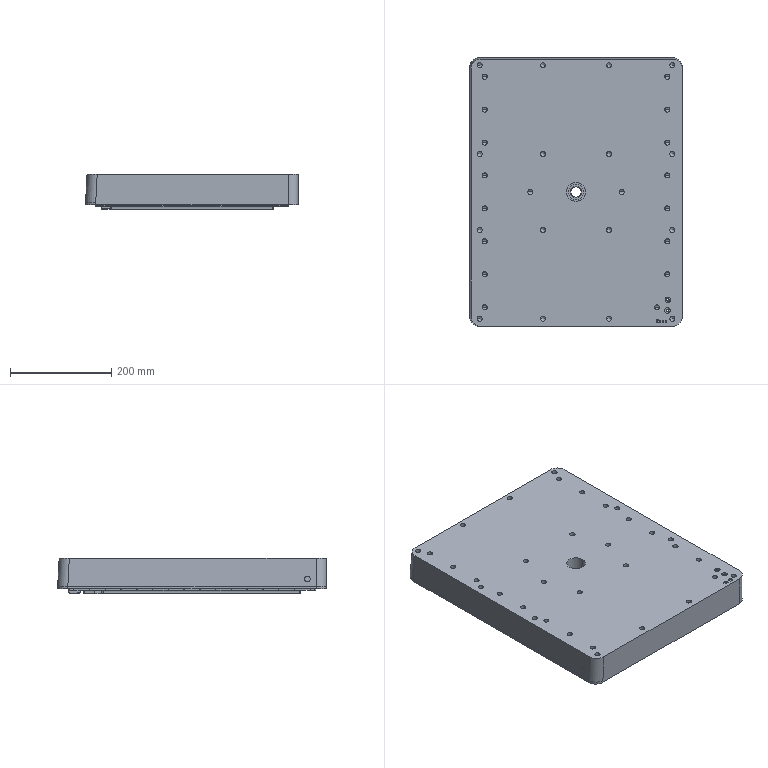Part | Creo | 1 solid | 689 faces | box 420 x 530 x 69.839 mm | volume 14277084 mm3 | plane 335 | cylinder 212 | cone 76 | other 42 | torus 16 | sphere 8 | commonest cylinder face diameters 10 x77 10.199 x32 10.2 x32 11.4 x18 4 x8 8 x8